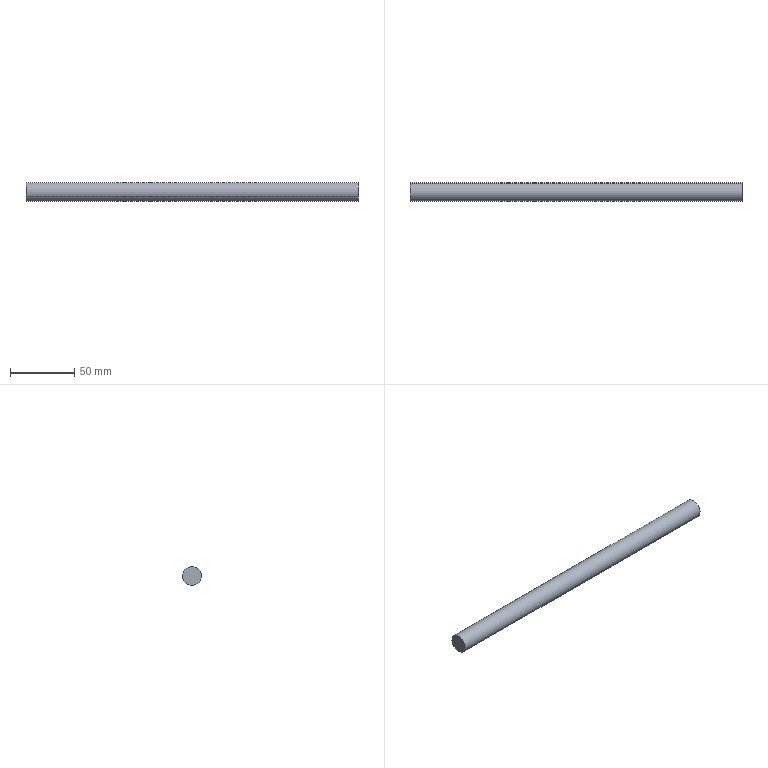Part | NX | 1 solid | 4 faces | box 258 x 14.64 x 14.64 mm | volume 43430 mm3 | cylinder 2 | plane 2 | commonest cylinder face diameters 14.64 x2
STEP:
#1=CARTESIAN_POINT('',(4.674,-534.907,2413.269));
#2=VERTEX_POINT('',#1);
#3=CARTESIAN_POINT('',(4.674,-548.091,2406.904));
#4=VERTEX_POINT('',#3);
#5=CARTESIAN_POINT('',(4.674,-541.499,2410.086));
#6=DIRECTION('',(1.,0.,0.));
#7=DIRECTION('',(0.,0.9005,0.4348));
#8=AXIS2_PLACEMENT_3D('',#5,#6,#7);
#9=CIRCLE('',#8,7.32);
#10=EDGE_CURVE('',#2,#4,#9,.T.);
#11=ORIENTED_EDGE('',*,*,#10,.F.);
#12=CARTESIAN_POINT('',(-253.326,-534.907,2413.269));
#13=VERTEX_POINT('',#12);
#14=CARTESIAN_POINT('',(4.674,-534.907,2413.269));
#15=DIRECTION('',(-1.,0.,0.));
#16=VECTOR('',#15,1.);
#17=LINE('',#14,#16);
#18=EDGE_CURVE('',#2,#13,#17,.T.);
#19=ORIENTED_EDGE('',*,*,#18,.T.);
#20=CARTESIAN_POINT('',(-253.326,-548.091,2406.904));
#21=VERTEX_POINT('',#20);
#22=CARTESIAN_POINT('',(-253.326,-541.499,2410.086));
#23=DIRECTION('',(-1.,0.,0.));
#24=DIRECTION('',(0.,-0.9005,-0.4348));
#25=AXIS2_PLACEMENT_3D('',#22,#23,#24);
#26=CIRCLE('',#25,7.32);
#27=EDGE_CURVE('',#21,#13,#26,.T.);
#28=ORIENTED_EDGE('',*,*,#27,.F.);
#29=CARTESIAN_POINT('',(4.674,-548.091,2406.904));
#30=DIRECTION('',(1.,0.,0.));
#31=VECTOR('',#30,1.);
#32=LINE('',#29,#31);
#33=EDGE_CURVE('',#21,#4,#32,.T.);
#34=ORIENTED_EDGE('',*,*,#33,.T.);
#35=EDGE_LOOP('',(#11,#19,#28,#34));
#36=FACE_OUTER_BOUND('',#35,.T.);
#37=CARTESIAN_POINT('',(4.674,-541.499,2410.086));
#38=DIRECTION('',(-1.,0.,0.));
#39=DIRECTION('',(0.,-0.9005,-0.4348));
#40=AXIS2_PLACEMENT_3D('',#37,#38,#39);
#41=CYLINDRICAL_SURFACE('',#40,7.32);
#42=ADVANCED_FACE('',(#36),#41,.T.);
#43=ORIENTED_EDGE('',*,*,#18,.F.);
#44=CARTESIAN_POINT('',(4.674,-541.499,2410.086));
#45=DIRECTION('',(1.,0.,0.));
#46=DIRECTION('',(0.,0.9005,0.4348));
#47=AXIS2_PLACEMENT_3D('',#44,#45,#46);
#48=CIRCLE('',#47,7.32);
#49=EDGE_CURVE('',#4,#2,#48,.T.);
#50=ORIENTED_EDGE('',*,*,#49,.F.);
#51=ORIENTED_EDGE('',*,*,#33,.F.);
#52=CARTESIAN_POINT('',(-253.326,-541.499,2410.086));
#53=DIRECTION('',(-1.,0.,0.));
#54=DIRECTION('',(0.,-0.9005,-0.4348));
#55=AXIS2_PLACEMENT_3D('',#52,#53,#54);
#56=CIRCLE('',#55,7.32);
#57=EDGE_CURVE('',#13,#21,#56,.T.);
#58=ORIENTED_EDGE('',*,*,#57,.F.);
#59=EDGE_LOOP('',(#43,#50,#51,#58));
#60=FACE_OUTER_BOUND('',#59,.T.);
#61=CARTESIAN_POINT('',(4.674,-541.499,2410.086));
#62=DIRECTION('',(-1.,0.,0.));
#63=DIRECTION('',(0.,-0.9005,-0.4348));
#64=AXIS2_PLACEMENT_3D('',#61,#62,#63);
#65=CYLINDRICAL_SURFACE('',#64,7.32);
#66=ADVANCED_FACE('',(#60),#65,.T.);
#67=ORIENTED_EDGE('',*,*,#49,.T.);
#68=ORIENTED_EDGE('',*,*,#10,.T.);
#69=EDGE_LOOP('',(#67,#68));
#70=FACE_OUTER_BOUND('',#69,.T.);
#71=CARTESIAN_POINT('',(4.674,-541.499,2410.086));
#72=DIRECTION('',(1.,0.,0.));
#73=DIRECTION('',(0.,0.9005,0.4348));
#74=AXIS2_PLACEMENT_3D('',#71,#72,#73);
#75=PLANE('',#74);
#76=ADVANCED_FACE('',(#70),#75,.T.);
#77=ORIENTED_EDGE('',*,*,#27,.T.);
#78=ORIENTED_EDGE('',*,*,#57,.T.);
#79=EDGE_LOOP('',(#77,#78));
#80=FACE_OUTER_BOUND('',#79,.T.);
#81=CARTESIAN_POINT('',(-253.326,-541.499,2410.086));
#82=DIRECTION('',(-1.,0.,0.));
#83=DIRECTION('',(0.,-0.9005,-0.4348));
#84=AXIS2_PLACEMENT_3D('',#81,#82,#83);
#85=PLANE('',#84);
#86=ADVANCED_FACE('',(#80),#85,.T.);
#87=CLOSED_SHELL('',(#42,#66,#76,#86));
#88=MANIFOLD_SOLID_BREP('',#87);
#89=(LENGTH_UNIT()NAMED_UNIT(*)SI_UNIT(.MILLI.,.METRE.));
#90=UNCERTAINTY_MEASURE_WITH_UNIT(LENGTH_MEASURE(0.00002),#89,'','');
#91=(NAMED_UNIT(*)PLANE_ANGLE_UNIT()SI_UNIT($,.RADIAN.));
#92=PLANE_ANGLE_MEASURE_WITH_UNIT(PLANE_ANGLE_MEASURE(0.01745),#91);
#93=DIMENSIONAL_EXPONENTS(0.,0.,0.,0.,0.,0.,0.);
#94=(CONVERSION_BASED_UNIT('DEGREE',#92)NAMED_UNIT(#93)PLANE_ANGLE_UNIT());
#95=(NAMED_UNIT(*)SI_UNIT($,.STERADIAN.)SOLID_ANGLE_UNIT());
#96=(GEOMETRIC_REPRESENTATION_CONTEXT(3)GLOBAL_UNCERTAINTY_ASSIGNED_CONTEXT((#90))GLOBAL_UNIT_ASSIGNED_CONTEXT((#89,#94,#95))REPRESENTATION_CONTEXT('',''));
#97=ADVANCED_BREP_SHAPE_REPRESENTATION('',(#88),#96);